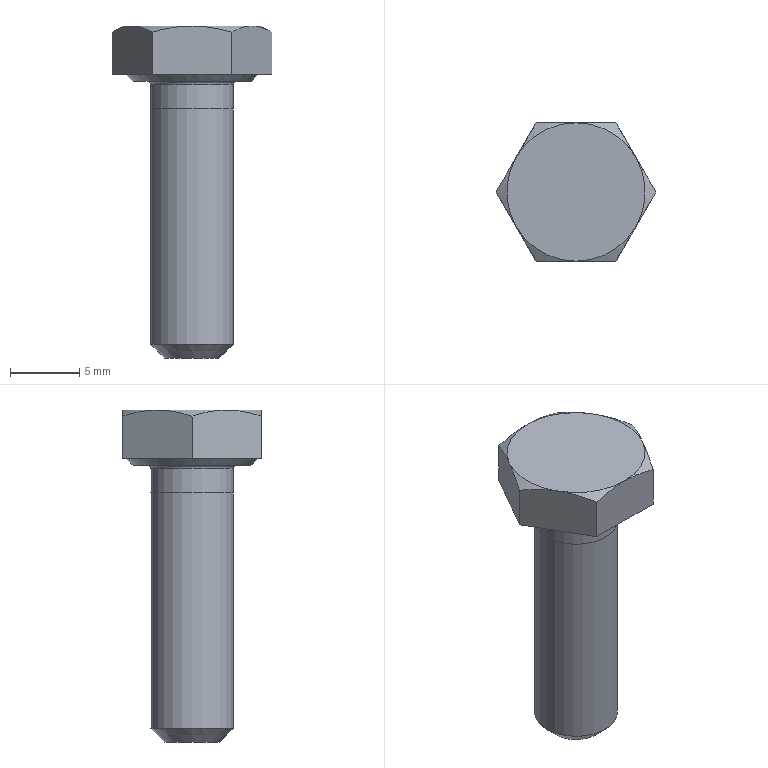Part | NX | features BREP 1, DATUM_CSYS 1 | 1 solid | 21 faces | box 11.547 x 10 x 24 mm | volume 891.515 mm3 | plane 10 | cone 8 | cylinder 2 | torus 1 | commonest cylinder face diameters 6 x2
STEP:
#1=CARTESIAN_POINT('',(4.33,2.5,4.));
#2=VERTEX_POINT('',#1);
#3=CARTESIAN_POINT('',(4.33,-2.5,4.));
#4=VERTEX_POINT('',#3);
#5=CARTESIAN_POINT('',(0.,0.,4.));
#6=DIRECTION('',(0.,0.,-1.));
#7=DIRECTION('',(0.866,0.5,0.));
#8=AXIS2_PLACEMENT_3D('',#5,#6,#7);
#9=CIRCLE('',#8,5.);
#10=EDGE_CURVE('',#2,#4,#9,.T.);
#11=ORIENTED_EDGE('',*,*,#10,.F.);
#12=CARTESIAN_POINT('',(0.000000002,5.,4.));
#13=VERTEX_POINT('',#12);
#14=CARTESIAN_POINT('',(0.,0.,4.));
#15=DIRECTION('',(0.,0.,1.));
#16=DIRECTION('',(0.866,0.5,0.));
#17=AXIS2_PLACEMENT_3D('',#14,#15,#16);
#18=CIRCLE('',#17,5.);
#19=EDGE_CURVE('',#2,#13,#18,.T.);
#20=ORIENTED_EDGE('',*,*,#19,.T.);
#21=CARTESIAN_POINT('',(-4.33,2.5,4.));
#22=VERTEX_POINT('',#21);
#23=CARTESIAN_POINT('',(0.,0.,4.));
#24=DIRECTION('',(0.,0.,1.));
#25=DIRECTION('',(0.,1.,0.));
#26=AXIS2_PLACEMENT_3D('',#23,#24,#25);
#27=CIRCLE('',#26,5.);
#28=EDGE_CURVE('',#13,#22,#27,.T.);
#29=ORIENTED_EDGE('',*,*,#28,.T.);
#30=CARTESIAN_POINT('',(-4.33,-2.5,4.));
#31=VERTEX_POINT('',#30);
#32=CARTESIAN_POINT('',(0.,0.,4.));
#33=DIRECTION('',(0.,0.,1.));
#34=DIRECTION('',(-0.866,0.5,0.));
#35=AXIS2_PLACEMENT_3D('',#32,#33,#34);
#36=CIRCLE('',#35,5.);
#37=EDGE_CURVE('',#22,#31,#36,.T.);
#38=ORIENTED_EDGE('',*,*,#37,.T.);
#39=CARTESIAN_POINT('',(-0.000000002,-5.,4.));
#40=VERTEX_POINT('',#39);
#41=CARTESIAN_POINT('',(0.,0.,4.));
#42=DIRECTION('',(0.,0.,1.));
#43=DIRECTION('',(-0.866,-0.5,0.));
#44=AXIS2_PLACEMENT_3D('',#41,#42,#43);
#45=CIRCLE('',#44,5.);
#46=EDGE_CURVE('',#31,#40,#45,.T.);
#47=ORIENTED_EDGE('',*,*,#46,.T.);
#48=CARTESIAN_POINT('',(0.,0.,4.));
#49=DIRECTION('',(0.,0.,1.));
#50=DIRECTION('',(0.,-1.,0.));
#51=AXIS2_PLACEMENT_3D('',#48,#49,#50);
#52=CIRCLE('',#51,5.);
#53=EDGE_CURVE('',#40,#4,#52,.T.);
#54=ORIENTED_EDGE('',*,*,#53,.T.);
#55=EDGE_LOOP('',(#11,#20,#29,#38,#47,#54));
#56=FACE_BOUND('',#55,.T.);
#57=CARTESIAN_POINT('',(0.,0.7735,4.));
#58=DIRECTION('',(0.,0.,1.));
#59=DIRECTION('',(-1.,0.,0.));
#60=AXIS2_PLACEMENT_3D('',#57,#58,#59);
#61=PLANE('',#60);
#62=ADVANCED_FACE('',(#56),#61,.T.);
#63=CARTESIAN_POINT('',(5.774,0.,0.5));
#64=VERTEX_POINT('',#63);
#65=CARTESIAN_POINT('',(2.887,5.,0.5));
#66=VERTEX_POINT('',#65);
#67=CARTESIAN_POINT('',(5.774,0.,0.5));
#68=DIRECTION('',(-0.5,0.866,0.));
#69=VECTOR('',#68,1000.);
#70=LINE('',#67,#69);
#71=EDGE_CURVE('',#64,#66,#70,.T.);
#72=ORIENTED_EDGE('',*,*,#71,.T.);
#73=CARTESIAN_POINT('',(2.887,5.,3.553));
#74=VERTEX_POINT('',#73);
#75=CARTESIAN_POINT('',(2.887,5.,0.5));
#76=DIRECTION('',(0.,0.,1.));
#77=VECTOR('',#76,1000.);
#78=LINE('',#75,#77);
#79=EDGE_CURVE('',#66,#74,#78,.T.);
#80=ORIENTED_EDGE('',*,*,#79,.T.);
#81=CARTESIAN_POINT('',(4.33,2.5,4.));
#82=CARTESIAN_POINT('',(3.66,3.66,4.));
#83=CARTESIAN_POINT('',(2.887,5.,3.553));
#84=(BOUNDED_CURVE()B_SPLINE_CURVE(2,(#81,#82,#83),.UNSPECIFIED.,.F.,.F.)B_SPLINE_CURVE_WITH_KNOTS((3,3),(0.,1.),.PIECEWISE_BEZIER_KNOTS.)CURVE()GEOMETRIC_REPRESENTATION_ITEM()RATIONAL_B_SPLINE_CURVE((1.544,1.544,1.434))REPRESENTATION_ITEM(''));
#85=EDGE_CURVE('',#2,#74,#84,.T.);
#86=ORIENTED_EDGE('',*,*,#85,.F.);
#87=CARTESIAN_POINT('',(5.774,0.,3.553));
#88=VERTEX_POINT('',#87);
#89=CARTESIAN_POINT('',(5.774,0.,3.553));
#90=CARTESIAN_POINT('',(5.,1.34,4.));
#91=CARTESIAN_POINT('',(4.33,2.5,4.));
#92=(BOUNDED_CURVE()B_SPLINE_CURVE(2,(#89,#90,#91),.UNSPECIFIED.,.F.,.F.)B_SPLINE_CURVE_WITH_KNOTS((3,3),(0.,1.),.PIECEWISE_BEZIER_KNOTS.)CURVE()GEOMETRIC_REPRESENTATION_ITEM()RATIONAL_B_SPLINE_CURVE((1.434,1.544,1.544))REPRESENTATION_ITEM(''));
#93=EDGE_CURVE('',#88,#2,#92,.T.);
#94=ORIENTED_EDGE('',*,*,#93,.F.);
#95=CARTESIAN_POINT('',(5.774,0.,0.5));
#96=DIRECTION('',(0.,0.,1.));
#97=VECTOR('',#96,1000.);
#98=LINE('',#95,#97);
#99=EDGE_CURVE('',#64,#88,#98,.T.);
#100=ORIENTED_EDGE('',*,*,#99,.F.);
#101=EDGE_LOOP('',(#72,#80,#86,#94,#100));
#102=FACE_BOUND('',#101,.T.);
#103=CARTESIAN_POINT('',(4.33,2.5,2.25));
#104=DIRECTION('',(0.866,0.5,0.));
#105=DIRECTION('',(0.5,-0.866,0.));
#106=AXIS2_PLACEMENT_3D('',#103,#104,#105);
#107=PLANE('',#106);
#108=ADVANCED_FACE('',(#102),#107,.T.);
#109=CARTESIAN_POINT('',(-2.887,5.,0.5));
#110=VERTEX_POINT('',#109);
#111=CARTESIAN_POINT('',(2.887,5.,0.5));
#112=DIRECTION('',(-1.,0.,0.));
#113=VECTOR('',#112,1000.);
#114=LINE('',#111,#113);
#115=EDGE_CURVE('',#66,#110,#114,.T.);
#116=ORIENTED_EDGE('',*,*,#115,.T.);
#117=CARTESIAN_POINT('',(-2.887,5.,3.553));
#118=VERTEX_POINT('',#117);
#119=CARTESIAN_POINT('',(-2.887,5.,0.5));
#120=DIRECTION('',(0.,0.,1.));
#121=VECTOR('',#120,1000.);
#122=LINE('',#119,#121);
#123=EDGE_CURVE('',#110,#118,#122,.T.);
#124=ORIENTED_EDGE('',*,*,#123,.T.);
#125=CARTESIAN_POINT('',(0.,5.,4.));
#126=CARTESIAN_POINT('',(-1.34,5.,4.));
#127=CARTESIAN_POINT('',(-2.887,5.,3.553));
#128=(BOUNDED_CURVE()B_SPLINE_CURVE(2,(#125,#126,#127),.UNSPECIFIED.,.F.,.F.)B_SPLINE_CURVE_WITH_KNOTS((3,3),(0.,1.),.PIECEWISE_BEZIER_KNOTS.)CURVE()GEOMETRIC_REPRESENTATION_ITEM()RATIONAL_B_SPLINE_CURVE((1.544,1.544,1.434))REPRESENTATION_ITEM(''));
#129=EDGE_CURVE('',#13,#118,#128,.T.);
#130=ORIENTED_EDGE('',*,*,#129,.F.);
#131=CARTESIAN_POINT('',(2.887,5.,3.553));
#132=CARTESIAN_POINT('',(1.34,5.,4.));
#133=CARTESIAN_POINT('',(0.000000004,5.,4.));
#134=(BOUNDED_CURVE()B_SPLINE_CURVE(2,(#131,#132,#133),.UNSPECIFIED.,.F.,.F.)B_SPLINE_CURVE_WITH_KNOTS((3,3),(0.,1.),.PIECEWISE_BEZIER_KNOTS.)CURVE()GEOMETRIC_REPRESENTATION_ITEM()RATIONAL_B_SPLINE_CURVE((1.434,1.544,1.544))REPRESENTATION_ITEM(''));
#135=EDGE_CURVE('',#74,#13,#134,.T.);
#136=ORIENTED_EDGE('',*,*,#135,.F.);
#137=ORIENTED_EDGE('',*,*,#79,.F.);
#138=EDGE_LOOP('',(#116,#124,#130,#136,#137));
#139=FACE_BOUND('',#138,.T.);
#140=CARTESIAN_POINT('',(0.,5.,2.25));
#141=DIRECTION('',(0.,1.,0.));
#142=DIRECTION('',(1.,0.,0.));
#143=AXIS2_PLACEMENT_3D('',#140,#141,#142);
#144=PLANE('',#143);
#145=ADVANCED_FACE('',(#139),#144,.T.);
#146=CARTESIAN_POINT('',(-5.774,0.,0.5));
#147=VERTEX_POINT('',#146);
#148=CARTESIAN_POINT('',(-2.887,5.,0.5));
#149=DIRECTION('',(-0.5,-0.866,0.));
#150=VECTOR('',#149,1000.);
#151=LINE('',#148,#150);
#152=EDGE_CURVE('',#110,#147,#151,.T.);
#153=ORIENTED_EDGE('',*,*,#152,.T.);
#154=CARTESIAN_POINT('',(-5.774,0.,3.553));
#155=VERTEX_POINT('',#154);
#156=CARTESIAN_POINT('',(-5.774,0.,0.5));
#157=DIRECTION('',(0.,0.,1.));
#158=VECTOR('',#157,1000.);
#159=LINE('',#156,#158);
#160=EDGE_CURVE('',#147,#155,#159,.T.);
#161=ORIENTED_EDGE('',*,*,#160,.T.);
#162=CARTESIAN_POINT('',(-4.33,2.5,4.));
#163=CARTESIAN_POINT('',(-5.,1.34,4.));
#164=CARTESIAN_POINT('',(-5.774,0.,3.553));
#165=(BOUNDED_CURVE()B_SPLINE_CURVE(2,(#162,#163,#164),.UNSPECIFIED.,.F.,.F.)B_SPLINE_CURVE_WITH_KNOTS((3,3),(0.,1.),.PIECEWISE_BEZIER_KNOTS.)CURVE()GEOMETRIC_REPRESENTATION_ITEM()RATIONAL_B_SPLINE_CURVE((1.544,1.544,1.434))REPRESENTATION_ITEM(''));
#166=EDGE_CURVE('',#22,#155,#165,.T.);
#167=ORIENTED_EDGE('',*,*,#166,.F.);
#168=CARTESIAN_POINT('',(-2.887,5.,3.553));
#169=CARTESIAN_POINT('',(-3.66,3.66,4.));
#170=CARTESIAN_POINT('',(-4.33,2.5,4.));
#171=(BOUNDED_CURVE()B_SPLINE_CURVE(2,(#168,#169,#170),.UNSPECIFIED.,.F.,.F.)B_SPLINE_CURVE_WITH_KNOTS((3,3),(0.,1.),.PIECEWISE_BEZIER_KNOTS.)CURVE()GEOMETRIC_REPRESENTATION_ITEM()RATIONAL_B_SPLINE_CURVE((1.434,1.544,1.544))REPRESENTATION_ITEM(''));
#172=EDGE_CURVE('',#118,#22,#171,.T.);
#173=ORIENTED_EDGE('',*,*,#172,.F.);
#174=ORIENTED_EDGE('',*,*,#123,.F.);
#175=EDGE_LOOP('',(#153,#161,#167,#173,#174));
#176=FACE_BOUND('',#175,.T.);
#177=CARTESIAN_POINT('',(-4.33,2.5,2.25));
#178=DIRECTION('',(-0.866,0.5,0.));
#179=DIRECTION('',(0.5,0.866,0.));
#180=AXIS2_PLACEMENT_3D('',#177,#178,#179);
#181=PLANE('',#180);
#182=ADVANCED_FACE('',(#176),#181,.T.);
#183=CARTESIAN_POINT('',(-2.887,-5.,0.5));
#184=VERTEX_POINT('',#183);
#185=CARTESIAN_POINT('',(-5.774,0.,0.5));
#186=DIRECTION('',(0.5,-0.866,0.));
#187=VECTOR('',#186,1000.);
#188=LINE('',#185,#187);
#189=EDGE_CURVE('',#147,#184,#188,.T.);
#190=ORIENTED_EDGE('',*,*,#189,.T.);
#191=CARTESIAN_POINT('',(-2.887,-5.,3.553));
#192=VERTEX_POINT('',#191);
#193=CARTESIAN_POINT('',(-2.887,-5.,0.5));
#194=DIRECTION('',(0.,0.,1.));
#195=VECTOR('',#194,1000.);
#196=LINE('',#193,#195);
#197=EDGE_CURVE('',#184,#192,#196,.T.);
#198=ORIENTED_EDGE('',*,*,#197,.T.);
#199=CARTESIAN_POINT('',(-4.33,-2.5,4.));
#200=CARTESIAN_POINT('',(-3.66,-3.66,4.));
#201=CARTESIAN_POINT('',(-2.887,-5.,3.553));
#202=(BOUNDED_CURVE()B_SPLINE_CURVE(2,(#199,#200,#201),.UNSPECIFIED.,.F.,.F.)B_SPLINE_CURVE_WITH_KNOTS((3,3),(0.,1.),.PIECEWISE_BEZIER_KNOTS.)CURVE()GEOMETRIC_REPRESENTATION_ITEM()RATIONAL_B_SPLINE_CURVE((1.544,1.544,1.434))REPRESENTATION_ITEM(''));
#203=EDGE_CURVE('',#31,#192,#202,.T.);
#204=ORIENTED_EDGE('',*,*,#203,.F.);
#205=CARTESIAN_POINT('',(-5.774,0.,3.553));
#206=CARTESIAN_POINT('',(-5.,-1.34,4.));
#207=CARTESIAN_POINT('',(-4.33,-2.5,4.));
#208=(BOUNDED_CURVE()B_SPLINE_CURVE(2,(#205,#206,#207),.UNSPECIFIED.,.F.,.F.)B_SPLINE_CURVE_WITH_KNOTS((3,3),(0.,1.),.PIECEWISE_BEZIER_KNOTS.)CURVE()GEOMETRIC_REPRESENTATION_ITEM()RATIONAL_B_SPLINE_CURVE((1.434,1.544,1.544))REPRESENTATION_ITEM(''));
#209=EDGE_CURVE('',#155,#31,#208,.T.);
#210=ORIENTED_EDGE('',*,*,#209,.F.);
#211=ORIENTED_EDGE('',*,*,#160,.F.);
#212=EDGE_LOOP('',(#190,#198,#204,#210,#211));
#213=FACE_BOUND('',#212,.T.);
#214=CARTESIAN_POINT('',(-4.33,-2.5,2.25));
#215=DIRECTION('',(-0.866,-0.5,0.));
#216=DIRECTION('',(-0.5,0.866,0.));
#217=AXIS2_PLACEMENT_3D('',#214,#215,#216);
#218=PLANE('',#217);
#219=ADVANCED_FACE('',(#213),#218,.T.);
#220=CARTESIAN_POINT('',(2.887,-5.,0.5));
#221=VERTEX_POINT('',#220);
#222=CARTESIAN_POINT('',(-2.887,-5.,0.5));
#223=DIRECTION('',(1.,0.,0.));
#224=VECTOR('',#223,1000.);
#225=LINE('',#222,#224);
#226=EDGE_CURVE('',#184,#221,#225,.T.);
#227=ORIENTED_EDGE('',*,*,#226,.T.);
#228=CARTESIAN_POINT('',(2.887,-5.,3.553));
#229=VERTEX_POINT('',#228);
#230=CARTESIAN_POINT('',(2.887,-5.,0.5));
#231=DIRECTION('',(0.,0.,1.));
#232=VECTOR('',#231,1000.);
#233=LINE('',#230,#232);
#234=EDGE_CURVE('',#221,#229,#233,.T.);
#235=ORIENTED_EDGE('',*,*,#234,.T.);
#236=CARTESIAN_POINT('',(0.,-5.,4.));
#237=CARTESIAN_POINT('',(1.34,-5.,4.));
#238=CARTESIAN_POINT('',(2.887,-5.,3.553));
#239=(BOUNDED_CURVE()B_SPLINE_CURVE(2,(#236,#237,#238),.UNSPECIFIED.,.F.,.F.)B_SPLINE_CURVE_WITH_KNOTS((3,3),(0.,1.),.PIECEWISE_BEZIER_KNOTS.)CURVE()GEOMETRIC_REPRESENTATION_ITEM()RATIONAL_B_SPLINE_CURVE((1.544,1.544,1.434))REPRESENTATION_ITEM(''));
#240=EDGE_CURVE('',#40,#229,#239,.T.);
#241=ORIENTED_EDGE('',*,*,#240,.F.);
#242=CARTESIAN_POINT('',(-2.887,-5.,3.553));
#243=CARTESIAN_POINT('',(-1.34,-5.,4.));
#244=CARTESIAN_POINT('',(-0.000000004,-5.,4.));
#245=(BOUNDED_CURVE()B_SPLINE_CURVE(2,(#242,#243,#244),.UNSPECIFIED.,.F.,.F.)B_SPLINE_CURVE_WITH_KNOTS((3,3),(0.,1.),.PIECEWISE_BEZIER_KNOTS.)CURVE()GEOMETRIC_REPRESENTATION_ITEM()RATIONAL_B_SPLINE_CURVE((1.434,1.544,1.544))REPRESENTATION_ITEM(''));
#246=EDGE_CURVE('',#192,#40,#245,.T.);
#247=ORIENTED_EDGE('',*,*,#246,.F.);
#248=ORIENTED_EDGE('',*,*,#197,.F.);
#249=EDGE_LOOP('',(#227,#235,#241,#247,#248));
#250=FACE_BOUND('',#249,.T.);
#251=CARTESIAN_POINT('',(0.,-5.,2.25));
#252=DIRECTION('',(0.,-1.,0.));
#253=DIRECTION('',(-1.,0.,0.));
#254=AXIS2_PLACEMENT_3D('',#251,#252,#253);
#255=PLANE('',#254);
#256=ADVANCED_FACE('',(#250),#255,.T.);
#257=CARTESIAN_POINT('',(2.887,-5.,0.5));
#258=DIRECTION('',(0.5,0.866,0.));
#259=VECTOR('',#258,1000.);
#260=LINE('',#257,#259);
#261=EDGE_CURVE('',#221,#64,#260,.T.);
#262=ORIENTED_EDGE('',*,*,#261,.T.);
#263=ORIENTED_EDGE('',*,*,#99,.T.);
#264=CARTESIAN_POINT('',(4.33,-2.5,4.));
#265=CARTESIAN_POINT('',(5.,-1.34,4.));
#266=CARTESIAN_POINT('',(5.774,0.,3.553));
#267=(BOUNDED_CURVE()B_SPLINE_CURVE(2,(#264,#265,#266),.UNSPECIFIED.,.F.,.F.)B_SPLINE_CURVE_WITH_KNOTS((3,3),(0.,1.),.PIECEWISE_BEZIER_KNOTS.)CURVE()GEOMETRIC_REPRESENTATION_ITEM()RATIONAL_B_SPLINE_CURVE((1.544,1.544,1.434))REPRESENTATION_ITEM(''));
#268=EDGE_CURVE('',#4,#88,#267,.T.);
#269=ORIENTED_EDGE('',*,*,#268,.F.);
#270=CARTESIAN_POINT('',(2.887,-5.,3.553));
#271=CARTESIAN_POINT('',(3.66,-3.66,4.));
#272=CARTESIAN_POINT('',(4.33,-2.5,4.));
#273=(BOUNDED_CURVE()B_SPLINE_CURVE(2,(#270,#271,#272),.UNSPECIFIED.,.F.,.F.)B_SPLINE_CURVE_WITH_KNOTS((3,3),(0.,1.),.PIECEWISE_BEZIER_KNOTS.)CURVE()GEOMETRIC_REPRESENTATION_ITEM()RATIONAL_B_SPLINE_CURVE((1.434,1.544,1.544))REPRESENTATION_ITEM(''));
#274=EDGE_CURVE('',#229,#4,#273,.T.);
#275=ORIENTED_EDGE('',*,*,#274,.F.);
#276=ORIENTED_EDGE('',*,*,#234,.F.);
#277=EDGE_LOOP('',(#262,#263,#269,#275,#276));
#278=FACE_BOUND('',#277,.T.);
#279=CARTESIAN_POINT('',(4.33,-2.5,2.25));
#280=DIRECTION('',(0.866,-0.5,0.));
#281=DIRECTION('',(-0.5,-0.866,0.));
#282=AXIS2_PLACEMENT_3D('',#279,#280,#281);
#283=PLANE('',#282);
#284=ADVANCED_FACE('',(#278),#283,.T.);
#285=ORIENTED_EDGE('',*,*,#261,.F.);
#286=ORIENTED_EDGE('',*,*,#226,.F.);
#287=ORIENTED_EDGE('',*,*,#189,.F.);
#288=ORIENTED_EDGE('',*,*,#152,.F.);
#289=ORIENTED_EDGE('',*,*,#115,.F.);
#290=ORIENTED_EDGE('',*,*,#71,.F.);
#291=EDGE_LOOP('',(#285,#286,#287,#288,#289,#290));
#292=FACE_BOUND('',#291,.T.);
#293=CARTESIAN_POINT('',(4.77,0.,0.5));
#294=VERTEX_POINT('',#293);
#295=CARTESIAN_POINT('',(0.,0.,0.5));
#296=DIRECTION('',(0.,0.,1.));
#297=DIRECTION('',(1.,0.,0.));
#298=AXIS2_PLACEMENT_3D('',#295,#296,#297);
#299=CIRCLE('',#298,4.77);
#300=EDGE_CURVE('',#294,#294,#299,.T.);
#301=ORIENTED_EDGE('',*,*,#300,.T.);
#302=EDGE_LOOP('',(#301));
#303=FACE_BOUND('',#302,.T.);
#304=CARTESIAN_POINT('',(0.,0.7735,0.5));
#305=DIRECTION('',(0.,0.,1.));
#306=DIRECTION('',(-1.,0.,0.));
#307=AXIS2_PLACEMENT_3D('',#304,#305,#306);
#308=PLANE('',#307);
#309=ADVANCED_FACE('',(#292,#303),#308,.F.);
#310=CARTESIAN_POINT('',(4.27,0.,0.));
#311=VERTEX_POINT('',#310);
#312=CARTESIAN_POINT('',(0.,0.,0.));
#313=DIRECTION('',(0.,0.,1.));
#314=DIRECTION('',(1.,0.,0.));
#315=AXIS2_PLACEMENT_3D('',#312,#313,#314);
#316=CIRCLE('',#315,4.27);
#317=EDGE_CURVE('',#311,#311,#316,.T.);
#318=ORIENTED_EDGE('',*,*,#317,.T.);
#319=CARTESIAN_POINT('',(4.27,0.,0.));
#320=DIRECTION('',(0.7071,0.,0.7071));
#321=VECTOR('',#320,1000.);
#322=LINE('',#319,#321);
#323=EDGE_CURVE('',#311,#294,#322,.T.);
#324=ORIENTED_EDGE('',*,*,#323,.T.);
#325=ORIENTED_EDGE('',*,*,#300,.F.);
#326=ORIENTED_EDGE('',*,*,#323,.F.);
#327=EDGE_LOOP('',(#318,#324,#325,#326));
#328=FACE_BOUND('',#327,.T.);
#329=CARTESIAN_POINT('',(0.,0.,0.));
#330=DIRECTION('',(0.,0.,1.));
#331=DIRECTION('',(-1.,0.,0.));
#332=AXIS2_PLACEMENT_3D('',#329,#330,#331);
#333=CONICAL_SURFACE('',#332,4.27,0.7854);
#334=ADVANCED_FACE('',(#328),#333,.T.);
#335=ORIENTED_EDGE('',*,*,#317,.F.);
#336=EDGE_LOOP('',(#335));
#337=FACE_BOUND('',#336,.T.);
#338=CARTESIAN_POINT('',(3.25,0.,0.));
#339=VERTEX_POINT('',#338);
#340=CARTESIAN_POINT('',(0.,0.,0.));
#341=DIRECTION('',(0.,0.,1.));
#342=DIRECTION('',(1.,0.,0.));
#343=AXIS2_PLACEMENT_3D('',#340,#341,#342);
#344=CIRCLE('',#343,3.25);
#345=EDGE_CURVE('',#339,#339,#344,.T.);
#346=ORIENTED_EDGE('',*,*,#345,.T.);
#347=EDGE_LOOP('',(#346));
#348=FACE_BOUND('',#347,.T.);
#349=CARTESIAN_POINT('',(0.,0.,0.));
#350=DIRECTION('',(0.,0.,1.));
#351=DIRECTION('',(-1.,0.,0.));
#352=AXIS2_PLACEMENT_3D('',#349,#350,#351);
#353=PLANE('',#352);
#354=ADVANCED_FACE('',(#337,#348),#353,.F.);
#355=CARTESIAN_POINT('',(3.,0.,-0.25));
#356=VERTEX_POINT('',#355);
#357=CARTESIAN_POINT('',(0.,0.,-0.25));
#358=DIRECTION('',(0.,0.,1.));
#359=DIRECTION('',(1.,0.,0.));
#360=AXIS2_PLACEMENT_3D('',#357,#358,#359);
#361=CIRCLE('',#360,3.);
#362=EDGE_CURVE('',#356,#356,#361,.T.);
#363=ORIENTED_EDGE('',*,*,#362,.T.);
#364=CARTESIAN_POINT('',(3.25,0.,-0.25));
#365=DIRECTION('',(0.,1.,0.));
#366=DIRECTION('',(-1.,0.,0.));
#367=AXIS2_PLACEMENT_3D('',#364,#365,#366);
#368=CIRCLE('',#367,0.25);
#369=EDGE_CURVE('',#356,#339,#368,.T.);
#370=ORIENTED_EDGE('',*,*,#369,.T.);
#371=ORIENTED_EDGE('',*,*,#345,.F.);
#372=ORIENTED_EDGE('',*,*,#369,.F.);
#373=EDGE_LOOP('',(#363,#370,#371,#372));
#374=FACE_BOUND('',#373,.T.);
#375=CARTESIAN_POINT('',(0.,0.,-0.25));
#376=DIRECTION('',(0.,0.,-1.));
#377=DIRECTION('',(-1.,0.,0.));
#378=AXIS2_PLACEMENT_3D('',#375,#376,#377);
#379=TOROIDAL_SURFACE('',#378,3.25,0.25);
#380=ADVANCED_FACE('',(#374),#379,.F.);
#381=CARTESIAN_POINT('',(3.,0.,-2.));
#382=VERTEX_POINT('',#381);
#383=CARTESIAN_POINT('',(0.,0.,-2.));
#384=DIRECTION('',(0.,0.,1.));
#385=DIRECTION('',(1.,0.,0.));
#386=AXIS2_PLACEMENT_3D('',#383,#384,#385);
#387=CIRCLE('',#386,3.);
#388=EDGE_CURVE('',#382,#382,#387,.T.);
#389=ORIENTED_EDGE('',*,*,#388,.T.);
#390=CARTESIAN_POINT('',(3.,0.,-2.));
#391=DIRECTION('',(0.,0.,1.));
#392=VECTOR('',#391,1000.);
#393=LINE('',#390,#392);
#394=EDGE_CURVE('',#382,#356,#393,.T.);
#395=ORIENTED_EDGE('',*,*,#394,.T.);
#396=ORIENTED_EDGE('',*,*,#362,.F.);
#397=ORIENTED_EDGE('',*,*,#394,.F.);
#398=EDGE_LOOP('',(#389,#395,#396,#397));
#399=FACE_BOUND('',#398,.T.);
#400=CARTESIAN_POINT('',(0.,0.,-2.));
#401=DIRECTION('',(0.,0.,1.));
#402=DIRECTION('',(-1.,0.,0.));
#403=AXIS2_PLACEMENT_3D('',#400,#401,#402);
#404=CYLINDRICAL_SURFACE('',#403,3.);
#405=ADVANCED_FACE('',(#399),#404,.T.);
#406=CARTESIAN_POINT('',(3.,0.,-19.));
#407=VERTEX_POINT('',#406);
#408=CARTESIAN_POINT('',(0.,0.,-19.));
#409=DIRECTION('',(0.,0.,1.));
#410=DIRECTION('',(1.,0.,0.));
#411=AXIS2_PLACEMENT_3D('',#408,#409,#410);
#412=CIRCLE('',#411,3.);
#413=EDGE_CURVE('',#407,#407,#412,.T.);
#414=ORIENTED_EDGE('',*,*,#413,.T.);
#415=CARTESIAN_POINT('',(3.,0.,-19.));
#416=DIRECTION('',(0.,0.,1.));
#417=VECTOR('',#416,1000.);
#418=LINE('',#415,#417);
#419=EDGE_CURVE('',#407,#382,#418,.T.);
#420=ORIENTED_EDGE('',*,*,#419,.T.);
#421=ORIENTED_EDGE('',*,*,#388,.F.);
#422=ORIENTED_EDGE('',*,*,#419,.F.);
#423=EDGE_LOOP('',(#414,#420,#421,#422));
#424=FACE_BOUND('',#423,.T.);
#425=CARTESIAN_POINT('',(0.,0.,-19.));
#426=DIRECTION('',(0.,0.,1.));
#427=DIRECTION('',(-1.,0.,0.));
#428=AXIS2_PLACEMENT_3D('',#425,#426,#427);
#429=CYLINDRICAL_SURFACE('',#428,3.);
#430=ADVANCED_FACE('',(#424),#429,.T.);
#431=CARTESIAN_POINT('',(2.,0.,-20.));
#432=VERTEX_POINT('',#431);
#433=CARTESIAN_POINT('',(0.,0.,-20.));
#434=DIRECTION('',(0.,0.,1.));
#435=DIRECTION('',(1.,0.,0.));
#436=AXIS2_PLACEMENT_3D('',#433,#434,#435);
#437=CIRCLE('',#436,2.);
#438=EDGE_CURVE('',#432,#432,#437,.T.);
#439=ORIENTED_EDGE('',*,*,#438,.T.);
#440=CARTESIAN_POINT('',(2.,0.,-20.));
#441=DIRECTION('',(0.7071,0.,0.7071));
#442=VECTOR('',#441,1000.);
#443=LINE('',#440,#442);
#444=EDGE_CURVE('',#432,#407,#443,.T.);
#445=ORIENTED_EDGE('',*,*,#444,.T.);
#446=ORIENTED_EDGE('',*,*,#413,.F.);
#447=ORIENTED_EDGE('',*,*,#444,.F.);
#448=EDGE_LOOP('',(#439,#445,#446,#447));
#449=FACE_BOUND('',#448,.T.);
#450=CARTESIAN_POINT('',(0.,0.,-20.));
#451=DIRECTION('',(0.,0.,1.));
#452=DIRECTION('',(-1.,0.,0.));
#453=AXIS2_PLACEMENT_3D('',#450,#451,#452);
#454=CONICAL_SURFACE('',#453,2.,0.7854);
#455=ADVANCED_FACE('',(#449),#454,.T.);
#456=ORIENTED_EDGE('',*,*,#438,.F.);
#457=EDGE_LOOP('',(#456));
#458=FACE_BOUND('',#457,.T.);
#459=CARTESIAN_POINT('',(0.,0.,-20.));
#460=DIRECTION('',(0.,0.,1.));
#461=DIRECTION('',(-1.,0.,0.));
#462=AXIS2_PLACEMENT_3D('',#459,#460,#461);
#463=PLANE('',#462);
#464=ADVANCED_FACE('',(#458),#463,.F.);
#465=ORIENTED_EDGE('',*,*,#19,.F.);
#466=ORIENTED_EDGE('',*,*,#85,.T.);
#467=ORIENTED_EDGE('',*,*,#135,.T.);
#468=EDGE_LOOP('',(#465,#466,#467));
#469=FACE_BOUND('',#468,.T.);
#470=CARTESIAN_POINT('',(0.,0.,4.));
#471=DIRECTION('',(0.,0.,-1.));
#472=DIRECTION('',(-0.9128,-0.4084,0.));
#473=AXIS2_PLACEMENT_3D('',#470,#471,#472);
#474=CONICAL_SURFACE('',#473,5.,1.047);
#475=ADVANCED_FACE('',(#469),#474,.T.);
#476=ORIENTED_EDGE('',*,*,#93,.T.);
#477=ORIENTED_EDGE('',*,*,#10,.T.);
#478=ORIENTED_EDGE('',*,*,#268,.T.);
#479=EDGE_LOOP('',(#476,#477,#478));
#480=FACE_BOUND('',#479,.T.);
#481=CARTESIAN_POINT('',(0.,0.,4.));
#482=DIRECTION('',(0.,0.,-1.));
#483=DIRECTION('',(-0.866,0.5,0.));
#484=AXIS2_PLACEMENT_3D('',#481,#482,#483);
#485=CONICAL_SURFACE('',#484,5.,1.047);
#486=ADVANCED_FACE('',(#480),#485,.T.);
#487=ORIENTED_EDGE('',*,*,#28,.F.);
#488=ORIENTED_EDGE('',*,*,#129,.T.);
#489=ORIENTED_EDGE('',*,*,#172,.T.);
#490=EDGE_LOOP('',(#487,#488,#489));
#491=FACE_BOUND('',#490,.T.);
#492=CARTESIAN_POINT('',(0.,0.,4.));
#493=DIRECTION('',(0.,0.,-1.));
#494=DIRECTION('',(-0.9128,-0.4084,0.));
#495=AXIS2_PLACEMENT_3D('',#492,#493,#494);
#496=CONICAL_SURFACE('',#495,5.,1.047);
#497=ADVANCED_FACE('',(#491),#496,.T.);
#498=ORIENTED_EDGE('',*,*,#37,.F.);
#499=ORIENTED_EDGE('',*,*,#166,.T.);
#500=ORIENTED_EDGE('',*,*,#209,.T.);
#501=EDGE_LOOP('',(#498,#499,#500));
#502=FACE_BOUND('',#501,.T.);
#503=CARTESIAN_POINT('',(0.,0.,4.));
#504=DIRECTION('',(0.,0.,-1.));
#505=DIRECTION('',(-0.9128,-0.4084,0.));
#506=AXIS2_PLACEMENT_3D('',#503,#504,#505);
#507=CONICAL_SURFACE('',#506,5.,1.047);
#508=ADVANCED_FACE('',(#502),#507,.T.);
#509=ORIENTED_EDGE('',*,*,#46,.F.);
#510=ORIENTED_EDGE('',*,*,#203,.T.);
#511=ORIENTED_EDGE('',*,*,#246,.T.);
#512=EDGE_LOOP('',(#509,#510,#511));
#513=FACE_BOUND('',#512,.T.);
#514=CARTESIAN_POINT('',(0.,0.,4.));
#515=DIRECTION('',(0.,0.,-1.));
#516=DIRECTION('',(-0.9128,-0.4084,0.));
#517=AXIS2_PLACEMENT_3D('',#514,#515,#516);
#518=CONICAL_SURFACE('',#517,5.,1.047);
#519=ADVANCED_FACE('',(#513),#518,.T.);
#520=ORIENTED_EDGE('',*,*,#53,.F.);
#521=ORIENTED_EDGE('',*,*,#240,.T.);
#522=ORIENTED_EDGE('',*,*,#274,.T.);
#523=EDGE_LOOP('',(#520,#521,#522));
#524=FACE_BOUND('',#523,.T.);
#525=CARTESIAN_POINT('',(0.,0.,4.));
#526=DIRECTION('',(0.,0.,-1.));
#527=DIRECTION('',(-0.9128,-0.4084,0.));
#528=AXIS2_PLACEMENT_3D('',#525,#526,#527);
#529=CONICAL_SURFACE('',#528,5.,1.047);
#530=ADVANCED_FACE('',(#524),#529,.T.);
#531=CLOSED_SHELL('',(#62,#108,#145,#182,#219,#256,#284,#309,#334,#354,#380,#405,#430,#455,#464,#475,#486,#497,#508,#519,#530));
#532=MANIFOLD_SOLID_BREP('',#531);
#533=(LENGTH_UNIT()NAMED_UNIT(*)SI_UNIT(.MILLI.,.METRE.));
#534=UNCERTAINTY_MEASURE_WITH_UNIT(LENGTH_MEASURE(0.00001),#533,'','');
#535=(NAMED_UNIT(*)PLANE_ANGLE_UNIT()SI_UNIT($,.RADIAN.));
#536=(NAMED_UNIT(*)SI_UNIT($,.STERADIAN.)SOLID_ANGLE_UNIT());
#537=(GEOMETRIC_REPRESENTATION_CONTEXT(3)GLOBAL_UNCERTAINTY_ASSIGNED_CONTEXT((#534))GLOBAL_UNIT_ASSIGNED_CONTEXT((#533,#535,#536))REPRESENTATION_CONTEXT('',''));
#538=ADVANCED_BREP_SHAPE_REPRESENTATION('',(#532),#537);